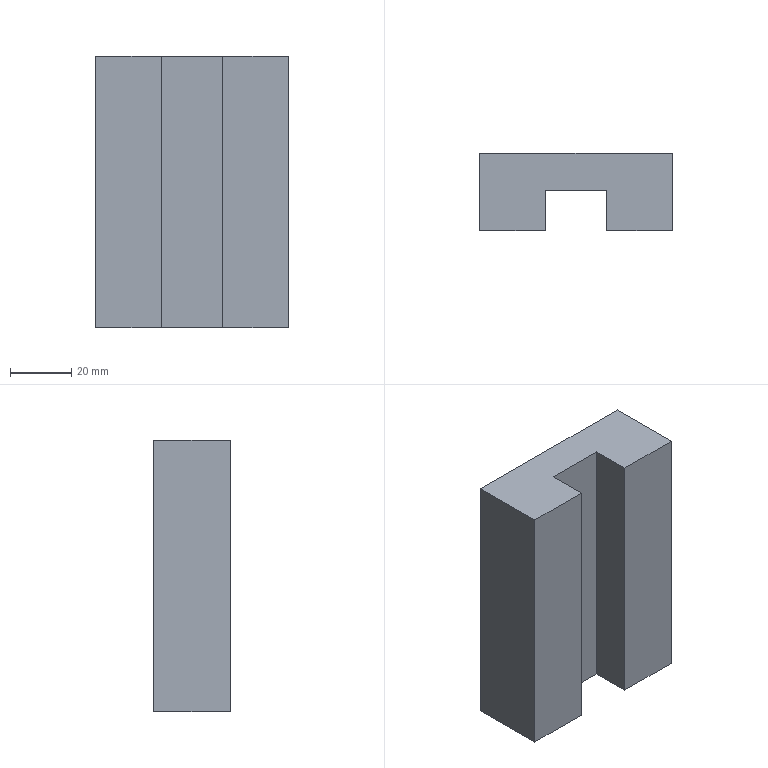Part | STEP file | MSA20LE slide seat | 1 solid | 26 faces | box 63 x 25 x 88.8 mm | volume 115397 mm3 | plane 10 | cylinder 8 | cone 8 | commonest cylinder face diameters 5 x8